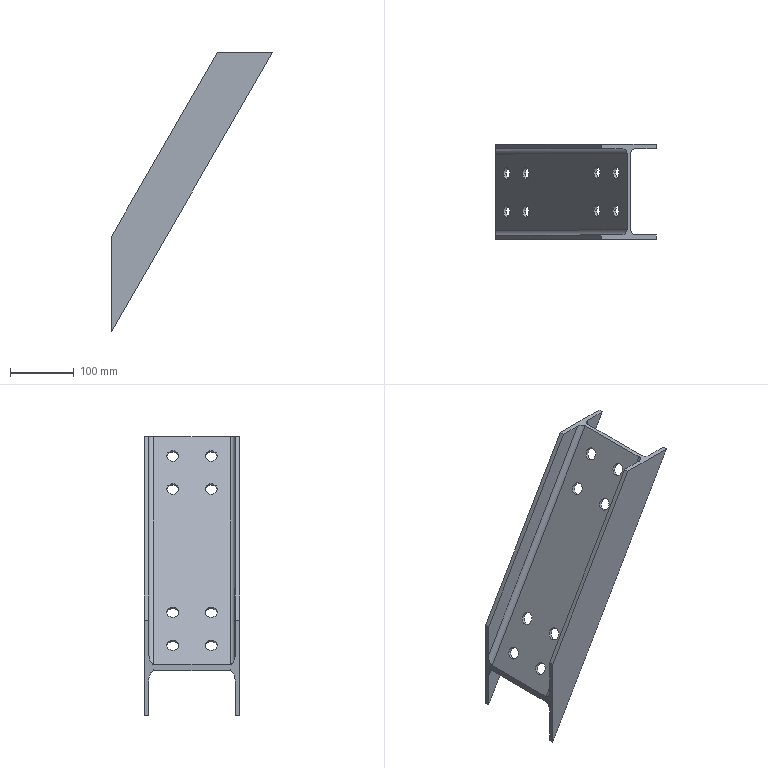Part | STEP file | 粉仓Diagonal Brace梁3-2_Default<As Machined> | 1 solid | 34 faces | box 253.301 x 150 x 438.731 mm | volume 738333 mm3 | cylinder 20 | plane 14 | commonest cylinder face diameters 19 x16 16 x4